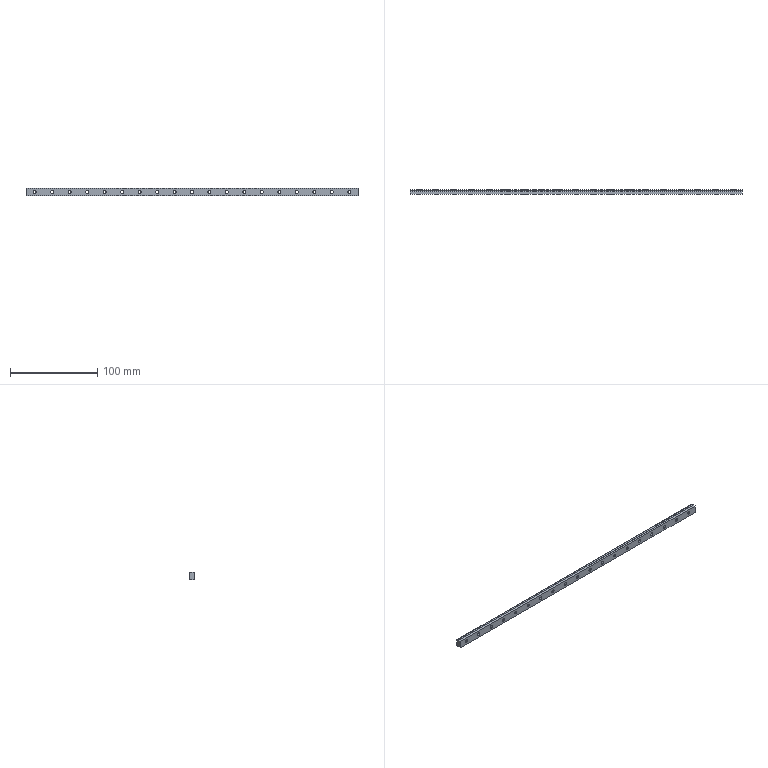Part | STEP file | RSR9KM1-500-1 | 1 solid | 69 faces | box 380 x 5.5 x 9 mm | volume 15608 mm3 | cylinder 40 | plane 29 | commonest cylinder face diameters 3.5 x19 6 x19 2 x2